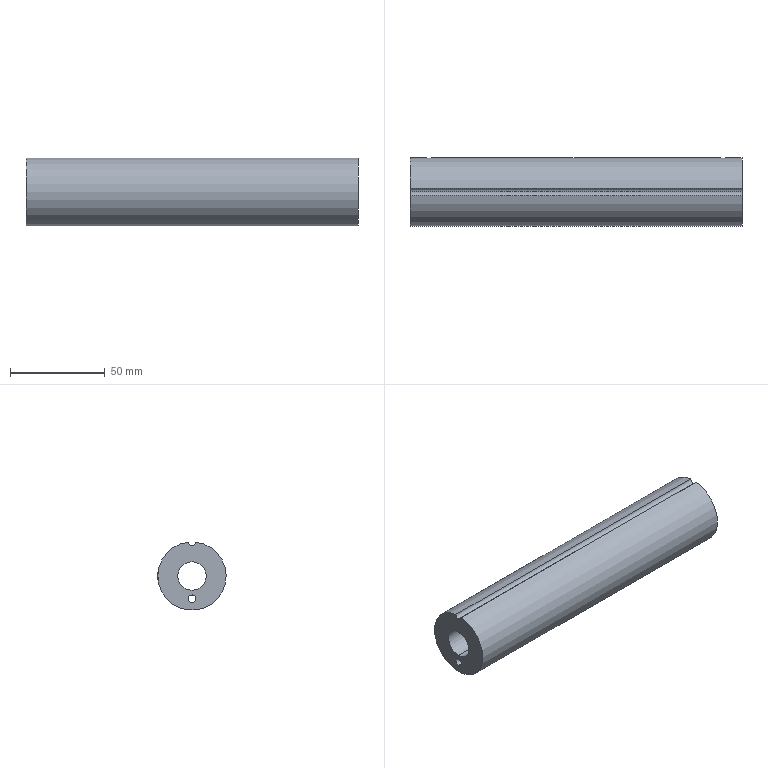Part | STEP file | MT-COMBO-119-S018 | 1 solid | 13 faces | box 175 x 36 x 35.889 mm | volume 143638 mm3 | cylinder 11 | plane 2 | commonest cylinder face diameters 4 x4 4.2 x4 15 x2 36 x1
STEP:
#1=CARTESIAN_POINT('',(-77.5,17.877,2.1));
#2=VERTEX_POINT('',#1);
#3=CARTESIAN_POINT('',(-77.5,17.877,-2.1));
#4=VERTEX_POINT('',#3);
#5=CARTESIAN_POINT('',(-77.5,17.877,2.1));
#6=CARTESIAN_POINT('',(-77.639,17.877,2.1));
#7=CARTESIAN_POINT('',(-77.775,17.879,2.086));
#8=CARTESIAN_POINT('',(-78.044,17.885,2.033));
#9=CARTESIAN_POINT('',(-78.177,17.889,1.993));
#10=CARTESIAN_POINT('',(-78.432,17.901,1.887));
#11=CARTESIAN_POINT('',(-78.552,17.908,1.823));
#12=CARTESIAN_POINT('',(-78.78,17.923,1.67));
#13=CARTESIAN_POINT('',(-78.888,17.931,1.582));
#14=CARTESIAN_POINT('',(-79.178,17.955,1.291));
#15=CARTESIAN_POINT('',(-79.335,17.971,1.057));
#16=CARTESIAN_POINT('',(-79.545,17.993,0.5521));
#17=CARTESIAN_POINT('',(-79.6,18.,0.2761));
#18=CARTESIAN_POINT('',(-79.6,18.,-0.1404));
#19=CARTESIAN_POINT('',(-79.586,17.998,-0.2769));
#20=CARTESIAN_POINT('',(-79.533,17.992,-0.5454));
#21=CARTESIAN_POINT('',(-79.492,17.988,-0.6788));
#22=CARTESIAN_POINT('',(-79.386,17.976,-0.9329));
#23=CARTESIAN_POINT('',(-79.322,17.97,-1.053));
#24=CARTESIAN_POINT('',(-79.169,17.955,-1.281));
#25=CARTESIAN_POINT('',(-79.081,17.947,-1.389));
#26=CARTESIAN_POINT('',(-78.79,17.923,-1.679));
#27=CARTESIAN_POINT('',(-78.556,17.906,-1.836));
#28=CARTESIAN_POINT('',(-78.051,17.884,-2.045));
#29=CARTESIAN_POINT('',(-77.774,17.877,-2.1));
#30=CARTESIAN_POINT('',(-77.5,17.877,-2.1));
#31=B_SPLINE_CURVE_WITH_KNOTS('',3,(#5,#6,#7,#8,#9,#10,#11,#12,#13,#14,#15,#16,#17,#18,#19,#20,#21,#22,#23,#24,#25,#26,#27,#28,#29,#30),.UNSPECIFIED.,.F.,.F.,(4,2,2,2,2,2,2,2,2,2,2,2,4),(0.009857,0.01027,0.01068,0.01109,0.0115,0.01232,0.01314,0.01355,0.01396,0.01437,0.01478,0.01561,0.01643),.UNSPECIFIED.);
#32=EDGE_CURVE('',#2,#4,#31,.T.);
#33=ORIENTED_EDGE('',*,*,#32,.F.);
#34=CARTESIAN_POINT('',(-77.5,7.2,2.1));
#35=VERTEX_POINT('',#34);
#36=CARTESIAN_POINT('',(-77.5,0.,2.1));
#37=DIRECTION('',(0.,-1.,0.));
#38=VECTOR('',#37,1000.);
#39=LINE('',#36,#38);
#40=EDGE_CURVE('',#2,#35,#39,.T.);
#41=ORIENTED_EDGE('',*,*,#40,.T.);
#42=CARTESIAN_POINT('',(-77.5,7.2,-2.1));
#43=VERTEX_POINT('',#42);
#44=CARTESIAN_POINT('',(-77.5,7.2,-2.1));
#45=CARTESIAN_POINT('',(-77.64,7.2,-2.1));
#46=CARTESIAN_POINT('',(-77.777,7.204,-2.086));
#47=CARTESIAN_POINT('',(-78.046,7.219,-2.032));
#48=CARTESIAN_POINT('',(-78.18,7.231,-1.992));
#49=CARTESIAN_POINT('',(-78.434,7.259,-1.886));
#50=CARTESIAN_POINT('',(-78.554,7.276,-1.822));
#51=CARTESIAN_POINT('',(-78.782,7.312,-1.669));
#52=CARTESIAN_POINT('',(-78.889,7.332,-1.581));
#53=CARTESIAN_POINT('',(-79.178,7.391,-1.292));
#54=CARTESIAN_POINT('',(-79.334,7.429,-1.059));
#55=CARTESIAN_POINT('',(-79.492,7.47,-0.68));
#56=CARTESIAN_POINT('',(-79.532,7.481,-0.5469));
#57=CARTESIAN_POINT('',(-79.586,7.496,-0.2754));
#58=CARTESIAN_POINT('',(-79.6,7.5,-0.1387));
#59=CARTESIAN_POINT('',(-79.6,7.5,0.1369));
#60=CARTESIAN_POINT('',(-79.586,7.496,0.2768));
#61=CARTESIAN_POINT('',(-79.532,7.481,0.5468));
#62=CARTESIAN_POINT('',(-79.492,7.47,0.678));
#63=CARTESIAN_POINT('',(-79.333,7.429,1.061));
#64=CARTESIAN_POINT('',(-79.179,7.391,1.291));
#65=CARTESIAN_POINT('',(-78.887,7.332,1.583));
#66=CARTESIAN_POINT('',(-78.782,7.312,1.669));
#67=CARTESIAN_POINT('',(-78.555,7.276,1.821));
#68=CARTESIAN_POINT('',(-78.432,7.259,1.887));
#69=CARTESIAN_POINT('',(-78.179,7.231,1.992));
#70=CARTESIAN_POINT('',(-78.048,7.22,2.032));
#71=CARTESIAN_POINT('',(-77.777,7.204,2.086));
#72=CARTESIAN_POINT('',(-77.637,7.2,2.1));
#73=CARTESIAN_POINT('',(-77.5,7.2,2.1));
#74=B_SPLINE_CURVE_WITH_KNOTS('',3,(#44,#45,#46,#47,#48,#49,#50,#51,#52,#53,#54,#55,#56,#57,#58,#59,#60,#61,#62,#63,#64,#65,#66,#67,#68,#69,#70,#71,#72,#73),.UNSPECIFIED.,.F.,.F.,(4,2,2,2,2,2,2,2,2,2,2,2,2,2,4),(0.,0.0004124,0.0008248,0.001237,0.00165,0.002474,0.002887,0.003299,0.003712,0.004124,0.004949,0.005361,0.005774,0.006186,0.006599),.UNSPECIFIED.);
#75=EDGE_CURVE('',#43,#35,#74,.T.);
#76=ORIENTED_EDGE('',*,*,#75,.F.);
#77=CARTESIAN_POINT('',(-77.5,0.,-2.1));
#78=DIRECTION('',(0.,-1.,0.));
#79=VECTOR('',#78,1000.);
#80=LINE('',#77,#79);
#81=EDGE_CURVE('',#4,#43,#80,.T.);
#82=ORIENTED_EDGE('',*,*,#81,.F.);
#83=EDGE_LOOP('',(#33,#41,#76,#82));
#84=FACE_OUTER_BOUND('',#83,.T.);
#85=CARTESIAN_POINT('',(-77.5,0.,0.));
#86=DIRECTION('',(0.,-1.,0.));
#87=DIRECTION('',(0.,0.,-1.));
#88=AXIS2_PLACEMENT_3D('',#85,#86,#87);
#89=CYLINDRICAL_SURFACE('',#88,2.1);
#90=ADVANCED_FACE('',(#84),#89,.F.);
#91=CARTESIAN_POINT('',(77.5,17.877,2.1));
#92=VERTEX_POINT('',#91);
#93=CARTESIAN_POINT('',(77.5,17.877,-2.1));
#94=VERTEX_POINT('',#93);
#95=CARTESIAN_POINT('',(77.5,17.877,2.1));
#96=CARTESIAN_POINT('',(77.361,17.877,2.1));
#97=CARTESIAN_POINT('',(77.225,17.879,2.086));
#98=CARTESIAN_POINT('',(76.956,17.885,2.033));
#99=CARTESIAN_POINT('',(76.823,17.889,1.993));
#100=CARTESIAN_POINT('',(76.568,17.901,1.887));
#101=CARTESIAN_POINT('',(76.448,17.908,1.823));
#102=CARTESIAN_POINT('',(76.22,17.923,1.67));
#103=CARTESIAN_POINT('',(76.112,17.931,1.582));
#104=CARTESIAN_POINT('',(75.822,17.955,1.291));
#105=CARTESIAN_POINT('',(75.665,17.971,1.057));
#106=CARTESIAN_POINT('',(75.455,17.993,0.5521));
#107=CARTESIAN_POINT('',(75.4,18.,0.2761));
#108=CARTESIAN_POINT('',(75.4,18.,-0.1404));
#109=CARTESIAN_POINT('',(75.414,17.998,-0.2769));
#110=CARTESIAN_POINT('',(75.467,17.992,-0.5454));
#111=CARTESIAN_POINT('',(75.508,17.988,-0.6788));
#112=CARTESIAN_POINT('',(75.614,17.976,-0.9329));
#113=CARTESIAN_POINT('',(75.678,17.97,-1.053));
#114=CARTESIAN_POINT('',(75.831,17.955,-1.281));
#115=CARTESIAN_POINT('',(75.919,17.947,-1.389));
#116=CARTESIAN_POINT('',(76.21,17.923,-1.679));
#117=CARTESIAN_POINT('',(76.444,17.906,-1.836));
#118=CARTESIAN_POINT('',(76.949,17.884,-2.045));
#119=CARTESIAN_POINT('',(77.226,17.877,-2.1));
#120=CARTESIAN_POINT('',(77.5,17.877,-2.1));
#121=B_SPLINE_CURVE_WITH_KNOTS('',3,(#95,#96,#97,#98,#99,#100,#101,#102,#103,#104,#105,#106,#107,#108,#109,#110,#111,#112,#113,#114,#115,#116,#117,#118,#119,#120),.UNSPECIFIED.,.F.,.F.,(4,2,2,2,2,2,2,2,2,2,2,2,4),(0.009857,0.01027,0.01068,0.01109,0.0115,0.01232,0.01314,0.01355,0.01396,0.01437,0.01478,0.01561,0.01643),.UNSPECIFIED.);
#122=EDGE_CURVE('',#92,#94,#121,.T.);
#123=ORIENTED_EDGE('',*,*,#122,.F.);
#124=CARTESIAN_POINT('',(77.5,7.2,2.1));
#125=VERTEX_POINT('',#124);
#126=CARTESIAN_POINT('',(77.5,0.,2.1));
#127=DIRECTION('',(0.,-1.,0.));
#128=VECTOR('',#127,1000.);
#129=LINE('',#126,#128);
#130=EDGE_CURVE('',#92,#125,#129,.T.);
#131=ORIENTED_EDGE('',*,*,#130,.T.);
#132=CARTESIAN_POINT('',(77.5,7.2,-2.1));
#133=VERTEX_POINT('',#132);
#134=CARTESIAN_POINT('',(77.5,7.2,-2.1));
#135=CARTESIAN_POINT('',(77.36,7.2,-2.1));
#136=CARTESIAN_POINT('',(77.223,7.204,-2.086));
#137=CARTESIAN_POINT('',(76.954,7.219,-2.032));
#138=CARTESIAN_POINT('',(76.82,7.231,-1.992));
#139=CARTESIAN_POINT('',(76.566,7.259,-1.886));
#140=CARTESIAN_POINT('',(76.446,7.276,-1.822));
#141=CARTESIAN_POINT('',(76.218,7.312,-1.669));
#142=CARTESIAN_POINT('',(76.111,7.332,-1.581));
#143=CARTESIAN_POINT('',(75.822,7.391,-1.292));
#144=CARTESIAN_POINT('',(75.666,7.429,-1.059));
#145=CARTESIAN_POINT('',(75.508,7.47,-0.68));
#146=CARTESIAN_POINT('',(75.468,7.481,-0.5469));
#147=CARTESIAN_POINT('',(75.414,7.496,-0.2754));
#148=CARTESIAN_POINT('',(75.4,7.5,-0.1387));
#149=CARTESIAN_POINT('',(75.4,7.5,0.1369));
#150=CARTESIAN_POINT('',(75.414,7.496,0.2768));
#151=CARTESIAN_POINT('',(75.468,7.481,0.5468));
#152=CARTESIAN_POINT('',(75.508,7.47,0.678));
#153=CARTESIAN_POINT('',(75.667,7.429,1.061));
#154=CARTESIAN_POINT('',(75.821,7.391,1.291));
#155=CARTESIAN_POINT('',(76.113,7.332,1.583));
#156=CARTESIAN_POINT('',(76.218,7.312,1.669));
#157=CARTESIAN_POINT('',(76.445,7.276,1.821));
#158=CARTESIAN_POINT('',(76.568,7.259,1.887));
#159=CARTESIAN_POINT('',(76.821,7.231,1.992));
#160=CARTESIAN_POINT('',(76.952,7.22,2.032));
#161=CARTESIAN_POINT('',(77.223,7.204,2.086));
#162=CARTESIAN_POINT('',(77.363,7.2,2.1));
#163=CARTESIAN_POINT('',(77.5,7.2,2.1));
#164=B_SPLINE_CURVE_WITH_KNOTS('',3,(#134,#135,#136,#137,#138,#139,#140,#141,#142,#143,#144,#145,#146,#147,#148,#149,#150,#151,#152,#153,#154,#155,#156,#157,#158,#159,#160,#161,#162,#163),.UNSPECIFIED.,.F.,.F.,(4,2,2,2,2,2,2,2,2,2,2,2,2,2,4),(0.,0.0004124,0.0008248,0.001237,0.00165,0.002474,0.002887,0.003299,0.003712,0.004124,0.004949,0.005361,0.005774,0.006186,0.006599),.UNSPECIFIED.);
#165=EDGE_CURVE('',#133,#125,#164,.T.);
#166=ORIENTED_EDGE('',*,*,#165,.F.);
#167=CARTESIAN_POINT('',(77.5,0.,-2.1));
#168=DIRECTION('',(0.,-1.,0.));
#169=VECTOR('',#168,1000.);
#170=LINE('',#167,#169);
#171=EDGE_CURVE('',#94,#133,#170,.T.);
#172=ORIENTED_EDGE('',*,*,#171,.F.);
#173=EDGE_LOOP('',(#123,#131,#166,#172));
#174=FACE_OUTER_BOUND('',#173,.T.);
#175=CARTESIAN_POINT('',(77.5,0.,0.));
#176=DIRECTION('',(0.,-1.,0.));
#177=DIRECTION('',(0.,0.,-1.));
#178=AXIS2_PLACEMENT_3D('',#175,#176,#177);
#179=CYLINDRICAL_SURFACE('',#178,2.1);
#180=ADVANCED_FACE('',(#174),#179,.F.);
#181=CARTESIAN_POINT('',(-87.5,0.,-10.));
#182=VERTEX_POINT('',#181);
#183=CARTESIAN_POINT('',(-87.5,0.,-14.));
#184=VERTEX_POINT('',#183);
#185=CARTESIAN_POINT('',(-87.5,0.,-12.));
#186=DIRECTION('',(1.,0.,0.));
#187=DIRECTION('',(0.,0.,-1.));
#188=AXIS2_PLACEMENT_3D('',#185,#186,#187);
#189=CIRCLE('',#188,2.);
#190=EDGE_CURVE('',#182,#184,#189,.T.);
#191=ORIENTED_EDGE('',*,*,#190,.F.);
#192=CARTESIAN_POINT('',(87.5,0.,-10.));
#193=VERTEX_POINT('',#192);
#194=CARTESIAN_POINT('',(87.5,0.,-10.));
#195=DIRECTION('',(1.,0.,0.));
#196=VECTOR('',#195,1000.);
#197=LINE('',#194,#196);
#198=EDGE_CURVE('',#182,#193,#197,.T.);
#199=ORIENTED_EDGE('',*,*,#198,.T.);
#200=CARTESIAN_POINT('',(87.5,0.,-14.));
#201=VERTEX_POINT('',#200);
#202=CARTESIAN_POINT('',(87.5,0.,-12.));
#203=DIRECTION('',(1.,0.,0.));
#204=DIRECTION('',(0.,0.,-1.));
#205=AXIS2_PLACEMENT_3D('',#202,#203,#204);
#206=CIRCLE('',#205,2.);
#207=EDGE_CURVE('',#193,#201,#206,.T.);
#208=ORIENTED_EDGE('',*,*,#207,.T.);
#209=CARTESIAN_POINT('',(87.5,0.,-14.));
#210=DIRECTION('',(1.,0.,0.));
#211=VECTOR('',#210,1000.);
#212=LINE('',#209,#211);
#213=EDGE_CURVE('',#184,#201,#212,.T.);
#214=ORIENTED_EDGE('',*,*,#213,.F.);
#215=EDGE_LOOP('',(#191,#199,#208,#214));
#216=FACE_OUTER_BOUND('',#215,.T.);
#217=CARTESIAN_POINT('',(87.5,0.,-12.));
#218=DIRECTION('',(1.,0.,0.));
#219=DIRECTION('',(0.,0.,-1.));
#220=AXIS2_PLACEMENT_3D('',#217,#218,#219);
#221=CYLINDRICAL_SURFACE('',#220,2.);
#222=ADVANCED_FACE('',(#216),#221,.F.);
#223=CARTESIAN_POINT('',(-87.5,0.,16.));
#224=VERTEX_POINT('',#223);
#225=CARTESIAN_POINT('',(-87.5,1.997,17.889));
#226=VERTEX_POINT('',#225);
#227=CARTESIAN_POINT('',(-87.5,0.,18.));
#228=DIRECTION('',(1.,0.,0.));
#229=DIRECTION('',(0.,0.,-1.));
#230=AXIS2_PLACEMENT_3D('',#227,#228,#229);
#231=CIRCLE('',#230,2.);
#232=EDGE_CURVE('',#224,#226,#231,.T.);
#233=ORIENTED_EDGE('',*,*,#232,.F.);
#234=CARTESIAN_POINT('',(87.5,0.,16.));
#235=VERTEX_POINT('',#234);
#236=CARTESIAN_POINT('',(87.5,0.,16.));
#237=DIRECTION('',(1.,0.,0.));
#238=VECTOR('',#237,1000.);
#239=LINE('',#236,#238);
#240=EDGE_CURVE('',#224,#235,#239,.T.);
#241=ORIENTED_EDGE('',*,*,#240,.T.);
#242=CARTESIAN_POINT('',(87.5,1.997,17.889));
#243=VERTEX_POINT('',#242);
#244=CARTESIAN_POINT('',(87.5,0.,18.));
#245=DIRECTION('',(-1.,0.,0.));
#246=DIRECTION('',(0.,0.,1.));
#247=AXIS2_PLACEMENT_3D('',#244,#245,#246);
#248=CIRCLE('',#247,2.);
#249=EDGE_CURVE('',#243,#235,#248,.T.);
#250=ORIENTED_EDGE('',*,*,#249,.F.);
#251=CARTESIAN_POINT('',(0.,1.997,17.889));
#252=DIRECTION('',(1.,0.,0.));
#253=VECTOR('',#252,1000.);
#254=LINE('',#251,#253);
#255=EDGE_CURVE('',#226,#243,#254,.T.);
#256=ORIENTED_EDGE('',*,*,#255,.F.);
#257=EDGE_LOOP('',(#233,#241,#250,#256));
#258=FACE_OUTER_BOUND('',#257,.T.);
#259=CARTESIAN_POINT('',(87.5,0.,18.));
#260=DIRECTION('',(1.,0.,0.));
#261=DIRECTION('',(0.,0.,-1.));
#262=AXIS2_PLACEMENT_3D('',#259,#260,#261);
#263=CYLINDRICAL_SURFACE('',#262,2.);
#264=ADVANCED_FACE('',(#258),#263,.F.);
#265=CARTESIAN_POINT('',(87.5,0.,-7.5));
#266=VERTEX_POINT('',#265);
#267=CARTESIAN_POINT('',(87.5,0.,7.5));
#268=VERTEX_POINT('',#267);
#269=CARTESIAN_POINT('',(87.5,0.,0.));
#270=DIRECTION('',(-1.,0.,0.));
#271=DIRECTION('',(0.,0.,1.));
#272=AXIS2_PLACEMENT_3D('',#269,#270,#271);
#273=CIRCLE('',#272,7.5);
#274=EDGE_CURVE('',#266,#268,#273,.T.);
#275=ORIENTED_EDGE('',*,*,#274,.F.);
#276=CARTESIAN_POINT('',(-87.5,0.,-7.5));
#277=VERTEX_POINT('',#276);
#278=CARTESIAN_POINT('',(0.,0.,-7.5));
#279=DIRECTION('',(-1.,0.,0.));
#280=VECTOR('',#279,1000.);
#281=LINE('',#278,#280);
#282=EDGE_CURVE('',#266,#277,#281,.T.);
#283=ORIENTED_EDGE('',*,*,#282,.T.);
#284=CARTESIAN_POINT('',(-87.5,0.,7.5));
#285=VERTEX_POINT('',#284);
#286=CARTESIAN_POINT('',(-87.5,0.,0.));
#287=DIRECTION('',(-1.,0.,0.));
#288=DIRECTION('',(0.,0.,1.));
#289=AXIS2_PLACEMENT_3D('',#286,#287,#288);
#290=CIRCLE('',#289,7.5);
#291=EDGE_CURVE('',#277,#285,#290,.T.);
#292=ORIENTED_EDGE('',*,*,#291,.T.);
#293=CARTESIAN_POINT('',(0.,0.,7.5));
#294=DIRECTION('',(-1.,0.,0.));
#295=VECTOR('',#294,1000.);
#296=LINE('',#293,#295);
#297=EDGE_CURVE('',#268,#285,#296,.T.);
#298=ORIENTED_EDGE('',*,*,#297,.F.);
#299=EDGE_LOOP('',(#275,#283,#292,#298));
#300=FACE_OUTER_BOUND('',#299,.T.);
#301=CARTESIAN_POINT('',(0.,0.,0.));
#302=DIRECTION('',(-1.,0.,0.));
#303=DIRECTION('',(0.,0.,1.));
#304=AXIS2_PLACEMENT_3D('',#301,#302,#303);
#305=CYLINDRICAL_SURFACE('',#304,7.5);
#306=ADVANCED_FACE('',(#300),#305,.F.);
#307=CARTESIAN_POINT('',(-77.5,17.877,-2.1));
#308=CARTESIAN_POINT('',(-77.363,17.877,-2.1));
#309=CARTESIAN_POINT('',(-77.224,17.879,-2.086));
#310=CARTESIAN_POINT('',(-76.954,17.885,-2.032));
#311=CARTESIAN_POINT('',(-76.823,17.889,-1.993));
#312=CARTESIAN_POINT('',(-76.569,17.901,-1.887));
#313=CARTESIAN_POINT('',(-76.446,17.908,-1.822));
#314=CARTESIAN_POINT('',(-76.219,17.923,-1.669));
#315=CARTESIAN_POINT('',(-76.113,17.931,-1.583));
#316=CARTESIAN_POINT('',(-75.917,17.947,-1.387));
#317=CARTESIAN_POINT('',(-75.83,17.955,-1.281));
#318=CARTESIAN_POINT('',(-75.678,17.97,-1.053));
#319=CARTESIAN_POINT('',(-75.612,17.976,-0.9303));
#320=CARTESIAN_POINT('',(-75.507,17.988,-0.676));
#321=CARTESIAN_POINT('',(-75.467,17.992,-0.545));
#322=CARTESIAN_POINT('',(-75.414,17.998,-0.2756));
#323=CARTESIAN_POINT('',(-75.4,18.,-0.1364));
#324=CARTESIAN_POINT('',(-75.4,18.,0.275));
#325=CARTESIAN_POINT('',(-75.455,17.993,0.5515));
#326=CARTESIAN_POINT('',(-75.665,17.971,1.057));
#327=CARTESIAN_POINT('',(-75.821,17.955,1.291));
#328=CARTESIAN_POINT('',(-76.112,17.931,1.582));
#329=CARTESIAN_POINT('',(-76.22,17.923,1.67));
#330=CARTESIAN_POINT('',(-76.448,17.908,1.823));
#331=CARTESIAN_POINT('',(-76.568,17.901,1.887));
#332=CARTESIAN_POINT('',(-76.823,17.889,1.993));
#333=CARTESIAN_POINT('',(-76.956,17.885,2.033));
#334=CARTESIAN_POINT('',(-77.225,17.879,2.086));
#335=CARTESIAN_POINT('',(-77.361,17.877,2.1));
#336=CARTESIAN_POINT('',(-77.5,17.877,2.1));
#337=B_SPLINE_CURVE_WITH_KNOTS('',3,(#307,#308,#309,#310,#311,#312,#313,#314,#315,#316,#317,#318,#319,#320,#321,#322,#323,#324,#325,#326,#327,#328,#329,#330,#331,#332,#333,#334,#335,#336),.UNSPECIFIED.,.F.,.F.,(4,2,2,2,2,2,2,2,2,2,2,2,2,2,4),(0.003286,0.003697,0.004108,0.004518,0.004929,0.00534,0.005751,0.006161,0.006572,0.007393,0.008215,0.008625,0.009036,0.009447,0.009857),.UNSPECIFIED.);
#338=EDGE_CURVE('',#4,#2,#337,.T.);
#339=ORIENTED_EDGE('',*,*,#338,.T.);
#340=ORIENTED_EDGE('',*,*,#32,.T.);
#341=EDGE_LOOP('',(#339,#340));
#342=FACE_BOUND('',#341,.T.);
#343=CARTESIAN_POINT('',(77.5,17.877,-2.1));
#344=CARTESIAN_POINT('',(77.637,17.877,-2.1));
#345=CARTESIAN_POINT('',(77.776,17.879,-2.086));
#346=CARTESIAN_POINT('',(78.046,17.885,-2.032));
#347=CARTESIAN_POINT('',(78.177,17.889,-1.993));
#348=CARTESIAN_POINT('',(78.431,17.901,-1.887));
#349=CARTESIAN_POINT('',(78.554,17.908,-1.822));
#350=CARTESIAN_POINT('',(78.781,17.923,-1.669));
#351=CARTESIAN_POINT('',(78.887,17.931,-1.583));
#352=CARTESIAN_POINT('',(79.083,17.947,-1.387));
#353=CARTESIAN_POINT('',(79.17,17.955,-1.281));
#354=CARTESIAN_POINT('',(79.322,17.97,-1.053));
#355=CARTESIAN_POINT('',(79.388,17.976,-0.9303));
#356=CARTESIAN_POINT('',(79.493,17.988,-0.676));
#357=CARTESIAN_POINT('',(79.533,17.992,-0.545));
#358=CARTESIAN_POINT('',(79.586,17.998,-0.2756));
#359=CARTESIAN_POINT('',(79.6,18.,-0.1364));
#360=CARTESIAN_POINT('',(79.6,18.,0.275));
#361=CARTESIAN_POINT('',(79.545,17.993,0.5515));
#362=CARTESIAN_POINT('',(79.335,17.971,1.057));
#363=CARTESIAN_POINT('',(79.179,17.955,1.291));
#364=CARTESIAN_POINT('',(78.888,17.931,1.582));
#365=CARTESIAN_POINT('',(78.78,17.923,1.67));
#366=CARTESIAN_POINT('',(78.552,17.908,1.823));
#367=CARTESIAN_POINT('',(78.432,17.901,1.887));
#368=CARTESIAN_POINT('',(78.177,17.889,1.993));
#369=CARTESIAN_POINT('',(78.044,17.885,2.033));
#370=CARTESIAN_POINT('',(77.775,17.879,2.086));
#371=CARTESIAN_POINT('',(77.639,17.877,2.1));
#372=CARTESIAN_POINT('',(77.5,17.877,2.1));
#373=B_SPLINE_CURVE_WITH_KNOTS('',3,(#343,#344,#345,#346,#347,#348,#349,#350,#351,#352,#353,#354,#355,#356,#357,#358,#359,#360,#361,#362,#363,#364,#365,#366,#367,#368,#369,#370,#371,#372),.UNSPECIFIED.,.F.,.F.,(4,2,2,2,2,2,2,2,2,2,2,2,2,2,4),(0.003286,0.003697,0.004108,0.004518,0.004929,0.00534,0.005751,0.006161,0.006572,0.007393,0.008215,0.008625,0.009036,0.009447,0.009857),.UNSPECIFIED.);
#374=EDGE_CURVE('',#94,#92,#373,.T.);
#375=ORIENTED_EDGE('',*,*,#374,.T.);
#376=ORIENTED_EDGE('',*,*,#122,.T.);
#377=EDGE_LOOP('',(#375,#376));
#378=FACE_BOUND('',#377,.T.);
#379=CARTESIAN_POINT('',(-87.5,-1.997,17.889));
#380=VERTEX_POINT('',#379);
#381=CARTESIAN_POINT('',(-87.5,0.,0.));
#382=DIRECTION('',(-1.,0.,0.));
#383=DIRECTION('',(0.,0.,1.));
#384=AXIS2_PLACEMENT_3D('',#381,#382,#383);
#385=CIRCLE('',#384,18.);
#386=EDGE_CURVE('',#226,#380,#385,.T.);
#387=ORIENTED_EDGE('',*,*,#386,.F.);
#388=ORIENTED_EDGE('',*,*,#255,.T.);
#389=CARTESIAN_POINT('',(87.5,-1.997,17.889));
#390=VERTEX_POINT('',#389);
#391=CARTESIAN_POINT('',(87.5,0.,0.));
#392=DIRECTION('',(-1.,0.,0.));
#393=DIRECTION('',(0.,0.,1.));
#394=AXIS2_PLACEMENT_3D('',#391,#392,#393);
#395=CIRCLE('',#394,18.);
#396=EDGE_CURVE('',#243,#390,#395,.T.);
#397=ORIENTED_EDGE('',*,*,#396,.T.);
#398=CARTESIAN_POINT('',(0.,-1.997,17.889));
#399=DIRECTION('',(-1.,0.,0.));
#400=VECTOR('',#399,1000.);
#401=LINE('',#398,#400);
#402=EDGE_CURVE('',#390,#380,#401,.T.);
#403=ORIENTED_EDGE('',*,*,#402,.T.);
#404=EDGE_LOOP('',(#387,#388,#397,#403));
#405=FACE_OUTER_BOUND('',#404,.T.);
#406=CARTESIAN_POINT('',(0.,0.,0.));
#407=DIRECTION('',(-1.,0.,0.));
#408=DIRECTION('',(0.,0.,1.));
#409=AXIS2_PLACEMENT_3D('',#406,#407,#408);
#410=CYLINDRICAL_SURFACE('',#409,18.);
#411=ADVANCED_FACE('',(#342,#378,#405),#410,.T.);
#412=CARTESIAN_POINT('',(-87.5,0.,-12.));
#413=DIRECTION('',(1.,0.,0.));
#414=DIRECTION('',(0.,0.,-1.));
#415=AXIS2_PLACEMENT_3D('',#412,#413,#414);
#416=CIRCLE('',#415,2.);
#417=EDGE_CURVE('',#184,#182,#416,.T.);
#418=ORIENTED_EDGE('',*,*,#417,.T.);
#419=ORIENTED_EDGE('',*,*,#190,.T.);
#420=EDGE_LOOP('',(#418,#419));
#421=FACE_BOUND('',#420,.T.);
#422=CARTESIAN_POINT('',(-87.5,0.,0.));
#423=DIRECTION('',(-1.,0.,0.));
#424=DIRECTION('',(0.,0.,1.));
#425=AXIS2_PLACEMENT_3D('',#422,#423,#424);
#426=CIRCLE('',#425,7.5);
#427=EDGE_CURVE('',#285,#277,#426,.T.);
#428=ORIENTED_EDGE('',*,*,#427,.F.);
#429=ORIENTED_EDGE('',*,*,#291,.F.);
#430=EDGE_LOOP('',(#428,#429));
#431=FACE_BOUND('',#430,.T.);
#432=ORIENTED_EDGE('',*,*,#386,.T.);
#433=CARTESIAN_POINT('',(-87.5,0.,18.));
#434=DIRECTION('',(1.,0.,0.));
#435=DIRECTION('',(0.,0.,-1.));
#436=AXIS2_PLACEMENT_3D('',#433,#434,#435);
#437=CIRCLE('',#436,2.);
#438=EDGE_CURVE('',#380,#224,#437,.T.);
#439=ORIENTED_EDGE('',*,*,#438,.T.);
#440=ORIENTED_EDGE('',*,*,#232,.T.);
#441=EDGE_LOOP('',(#432,#439,#440));
#442=FACE_OUTER_BOUND('',#441,.T.);
#443=CARTESIAN_POINT('',(-87.5,18.,0.));
#444=DIRECTION('',(1.,0.,0.));
#445=DIRECTION('',(0.,0.,-1.));
#446=AXIS2_PLACEMENT_3D('',#443,#444,#445);
#447=PLANE('',#446);
#448=ADVANCED_FACE('',(#421,#431,#442),#447,.F.);
#449=ORIENTED_EDGE('',*,*,#282,.F.);
#450=CARTESIAN_POINT('',(87.5,0.,0.));
#451=DIRECTION('',(-1.,0.,0.));
#452=DIRECTION('',(0.,0.,1.));
#453=AXIS2_PLACEMENT_3D('',#450,#451,#452);
#454=CIRCLE('',#453,7.5);
#455=EDGE_CURVE('',#268,#266,#454,.T.);
#456=ORIENTED_EDGE('',*,*,#455,.F.);
#457=ORIENTED_EDGE('',*,*,#297,.T.);
#458=ORIENTED_EDGE('',*,*,#427,.T.);
#459=EDGE_LOOP('',(#449,#456,#457,#458));
#460=FACE_OUTER_BOUND('',#459,.T.);
#461=ORIENTED_EDGE('',*,*,#75,.T.);
#462=CARTESIAN_POINT('',(-77.5,7.2,2.1));
#463=CARTESIAN_POINT('',(-77.225,7.2,2.1));
#464=CARTESIAN_POINT('',(-76.948,7.217,2.044));
#465=CARTESIAN_POINT('',(-76.568,7.259,1.887));
#466=CARTESIAN_POINT('',(-76.445,7.276,1.821));
#467=CARTESIAN_POINT('',(-76.218,7.312,1.669));
#468=CARTESIAN_POINT('',(-76.113,7.332,1.582));
#469=CARTESIAN_POINT('',(-75.919,7.371,1.389));
#470=CARTESIAN_POINT('',(-75.831,7.391,1.282));
#471=CARTESIAN_POINT('',(-75.679,7.426,1.055));
#472=CARTESIAN_POINT('',(-75.614,7.443,0.9346));
#473=CARTESIAN_POINT('',(-75.508,7.47,0.6786));
#474=CARTESIAN_POINT('',(-75.468,7.481,0.547));
#475=CARTESIAN_POINT('',(-75.414,7.496,0.278));
#476=CARTESIAN_POINT('',(-75.4,7.5,0.1388));
#477=CARTESIAN_POINT('',(-75.4,7.5,-0.1381));
#478=CARTESIAN_POINT('',(-75.414,7.496,-0.2749));
#479=CARTESIAN_POINT('',(-75.467,7.481,-0.5451));
#480=CARTESIAN_POINT('',(-75.508,7.47,-0.6791));
#481=CARTESIAN_POINT('',(-75.666,7.429,-1.059));
#482=CARTESIAN_POINT('',(-75.822,7.391,-1.292));
#483=CARTESIAN_POINT('',(-76.111,7.332,-1.581));
#484=CARTESIAN_POINT('',(-76.218,7.312,-1.669));
#485=CARTESIAN_POINT('',(-76.446,7.276,-1.821));
#486=CARTESIAN_POINT('',(-76.566,7.259,-1.886));
#487=CARTESIAN_POINT('',(-76.819,7.231,-1.991));
#488=CARTESIAN_POINT('',(-76.953,7.219,-2.032));
#489=CARTESIAN_POINT('',(-77.223,7.204,-2.086));
#490=CARTESIAN_POINT('',(-77.361,7.2,-2.1));
#491=CARTESIAN_POINT('',(-77.5,7.2,-2.1));
#492=B_SPLINE_CURVE_WITH_KNOTS('',3,(#462,#463,#464,#465,#466,#467,#468,#469,#470,#471,#472,#473,#474,#475,#476,#477,#478,#479,#480,#481,#482,#483,#484,#485,#486,#487,#488,#489,#490,#491),.UNSPECIFIED.,.F.,.F.,(4,2,2,2,2,2,2,2,2,2,2,2,2,2,4),(0.006599,0.007423,0.007836,0.008248,0.00866,0.009072,0.009485,0.009897,0.01031,0.01072,0.01155,0.01196,0.01237,0.01278,0.0132),.UNSPECIFIED.);
#493=EDGE_CURVE('',#35,#43,#492,.T.);
#494=ORIENTED_EDGE('',*,*,#493,.T.);
#495=EDGE_LOOP('',(#461,#494));
#496=FACE_BOUND('',#495,.T.);
#497=ORIENTED_EDGE('',*,*,#165,.T.);
#498=CARTESIAN_POINT('',(77.5,7.2,2.1));
#499=CARTESIAN_POINT('',(77.775,7.2,2.1));
#500=CARTESIAN_POINT('',(78.052,7.217,2.044));
#501=CARTESIAN_POINT('',(78.432,7.259,1.887));
#502=CARTESIAN_POINT('',(78.555,7.276,1.821));
#503=CARTESIAN_POINT('',(78.782,7.312,1.669));
#504=CARTESIAN_POINT('',(78.887,7.332,1.582));
#505=CARTESIAN_POINT('',(79.081,7.371,1.389));
#506=CARTESIAN_POINT('',(79.169,7.391,1.282));
#507=CARTESIAN_POINT('',(79.321,7.426,1.055));
#508=CARTESIAN_POINT('',(79.386,7.443,0.9346));
#509=CARTESIAN_POINT('',(79.492,7.47,0.6786));
#510=CARTESIAN_POINT('',(79.532,7.481,0.547));
#511=CARTESIAN_POINT('',(79.586,7.496,0.278));
#512=CARTESIAN_POINT('',(79.6,7.5,0.1388));
#513=CARTESIAN_POINT('',(79.6,7.5,-0.1381));
#514=CARTESIAN_POINT('',(79.586,7.496,-0.2749));
#515=CARTESIAN_POINT('',(79.533,7.481,-0.5451));
#516=CARTESIAN_POINT('',(79.492,7.47,-0.6791));
#517=CARTESIAN_POINT('',(79.334,7.429,-1.059));
#518=CARTESIAN_POINT('',(79.178,7.391,-1.292));
#519=CARTESIAN_POINT('',(78.889,7.332,-1.581));
#520=CARTESIAN_POINT('',(78.782,7.312,-1.669));
#521=CARTESIAN_POINT('',(78.554,7.276,-1.821));
#522=CARTESIAN_POINT('',(78.434,7.259,-1.886));
#523=CARTESIAN_POINT('',(78.181,7.231,-1.991));
#524=CARTESIAN_POINT('',(78.047,7.219,-2.032));
#525=CARTESIAN_POINT('',(77.777,7.204,-2.086));
#526=CARTESIAN_POINT('',(77.639,7.2,-2.1));
#527=CARTESIAN_POINT('',(77.5,7.2,-2.1));
#528=B_SPLINE_CURVE_WITH_KNOTS('',3,(#498,#499,#500,#501,#502,#503,#504,#505,#506,#507,#508,#509,#510,#511,#512,#513,#514,#515,#516,#517,#518,#519,#520,#521,#522,#523,#524,#525,#526,#527),.UNSPECIFIED.,.F.,.F.,(4,2,2,2,2,2,2,2,2,2,2,2,2,2,4),(0.006599,0.007423,0.007836,0.008248,0.00866,0.009072,0.009485,0.009897,0.01031,0.01072,0.01155,0.01196,0.01237,0.01278,0.0132),.UNSPECIFIED.);
#529=EDGE_CURVE('',#125,#133,#528,.T.);
#530=ORIENTED_EDGE('',*,*,#529,.T.);
#531=EDGE_LOOP('',(#497,#530));
#532=FACE_BOUND('',#531,.T.);
#533=CARTESIAN_POINT('',(0.,0.,0.));
#534=DIRECTION('',(-1.,0.,0.));
#535=DIRECTION('',(0.,0.,1.));
#536=AXIS2_PLACEMENT_3D('',#533,#534,#535);
#537=CYLINDRICAL_SURFACE('',#536,7.5);
#538=ADVANCED_FACE('',(#460,#496,#532),#537,.F.);
#539=CARTESIAN_POINT('',(87.5,0.,-12.));
#540=DIRECTION('',(1.,0.,0.));
#541=DIRECTION('',(0.,0.,-1.));
#542=AXIS2_PLACEMENT_3D('',#539,#540,#541);
#543=CIRCLE('',#542,2.);
#544=EDGE_CURVE('',#201,#193,#543,.T.);
#545=ORIENTED_EDGE('',*,*,#544,.F.);
#546=ORIENTED_EDGE('',*,*,#207,.F.);
#547=EDGE_LOOP('',(#545,#546));
#548=FACE_BOUND('',#547,.T.);
#549=ORIENTED_EDGE('',*,*,#396,.F.);
#550=ORIENTED_EDGE('',*,*,#249,.T.);
#551=CARTESIAN_POINT('',(87.5,0.,18.));
#552=DIRECTION('',(-1.,0.,0.));
#553=DIRECTION('',(0.,0.,1.));
#554=AXIS2_PLACEMENT_3D('',#551,#552,#553);
#555=CIRCLE('',#554,2.);
#556=EDGE_CURVE('',#235,#390,#555,.T.);
#557=ORIENTED_EDGE('',*,*,#556,.T.);
#558=EDGE_LOOP('',(#549,#550,#557));
#559=FACE_OUTER_BOUND('',#558,.T.);
#560=ORIENTED_EDGE('',*,*,#455,.T.);
#561=ORIENTED_EDGE('',*,*,#274,.T.);
#562=EDGE_LOOP('',(#560,#561));
#563=FACE_BOUND('',#562,.T.);
#564=CARTESIAN_POINT('',(87.5,7.5,0.));
#565=DIRECTION('',(-1.,0.,0.));
#566=DIRECTION('',(0.,0.,1.));
#567=AXIS2_PLACEMENT_3D('',#564,#565,#566);
#568=PLANE('',#567);
#569=ADVANCED_FACE('',(#548,#559,#563),#568,.F.);
#570=ORIENTED_EDGE('',*,*,#240,.F.);
#571=ORIENTED_EDGE('',*,*,#438,.F.);
#572=ORIENTED_EDGE('',*,*,#402,.F.);
#573=ORIENTED_EDGE('',*,*,#556,.F.);
#574=EDGE_LOOP('',(#570,#571,#572,#573));
#575=FACE_OUTER_BOUND('',#574,.T.);
#576=CARTESIAN_POINT('',(87.5,0.,18.));
#577=DIRECTION('',(1.,0.,0.));
#578=DIRECTION('',(0.,0.,-1.));
#579=AXIS2_PLACEMENT_3D('',#576,#577,#578);
#580=CYLINDRICAL_SURFACE('',#579,2.);
#581=ADVANCED_FACE('',(#575),#580,.F.);
#582=ORIENTED_EDGE('',*,*,#198,.F.);
#583=ORIENTED_EDGE('',*,*,#417,.F.);
#584=ORIENTED_EDGE('',*,*,#213,.T.);
#585=ORIENTED_EDGE('',*,*,#544,.T.);
#586=EDGE_LOOP('',(#582,#583,#584,#585));
#587=FACE_OUTER_BOUND('',#586,.T.);
#588=CARTESIAN_POINT('',(87.5,0.,-12.));
#589=DIRECTION('',(1.,0.,0.));
#590=DIRECTION('',(0.,0.,-1.));
#591=AXIS2_PLACEMENT_3D('',#588,#589,#590);
#592=CYLINDRICAL_SURFACE('',#591,2.);
#593=ADVANCED_FACE('',(#587),#592,.F.);
#594=ORIENTED_EDGE('',*,*,#130,.F.);
#595=ORIENTED_EDGE('',*,*,#374,.F.);
#596=ORIENTED_EDGE('',*,*,#171,.T.);
#597=ORIENTED_EDGE('',*,*,#529,.F.);
#598=EDGE_LOOP('',(#594,#595,#596,#597));
#599=FACE_OUTER_BOUND('',#598,.T.);
#600=CARTESIAN_POINT('',(77.5,0.,0.));
#601=DIRECTION('',(0.,-1.,0.));
#602=DIRECTION('',(0.,0.,-1.));
#603=AXIS2_PLACEMENT_3D('',#600,#601,#602);
#604=CYLINDRICAL_SURFACE('',#603,2.1);
#605=ADVANCED_FACE('',(#599),#604,.F.);
#606=ORIENTED_EDGE('',*,*,#40,.F.);
#607=ORIENTED_EDGE('',*,*,#338,.F.);
#608=ORIENTED_EDGE('',*,*,#81,.T.);
#609=ORIENTED_EDGE('',*,*,#493,.F.);
#610=EDGE_LOOP('',(#606,#607,#608,#609));
#611=FACE_OUTER_BOUND('',#610,.T.);
#612=CARTESIAN_POINT('',(-77.5,0.,0.));
#613=DIRECTION('',(0.,-1.,0.));
#614=DIRECTION('',(0.,0.,-1.));
#615=AXIS2_PLACEMENT_3D('',#612,#613,#614);
#616=CYLINDRICAL_SURFACE('',#615,2.1);
#617=ADVANCED_FACE('',(#611),#616,.F.);
#618=CLOSED_SHELL('',(#90,#180,#222,#264,#306,#411,#448,#538,#569,#581,#593,#605,#617));
#619=MANIFOLD_SOLID_BREP('',#618);
#620=CARTESIAN_POINT('',(0.,0.,0.));
#621=DIRECTION('',(0.,0.,1.));
#622=DIRECTION('',(1.,0.,0.));
#623=AXIS2_PLACEMENT_3D('',#620,#621,#622);
#624=(LENGTH_UNIT()NAMED_UNIT(*)SI_UNIT(.MILLI.,.METRE.));
#625=UNCERTAINTY_MEASURE_WITH_UNIT(LENGTH_MEASURE(0.00001),#624,'','');
#626=(NAMED_UNIT(*)PLANE_ANGLE_UNIT()SI_UNIT($,.RADIAN.));
#627=(NAMED_UNIT(*)SI_UNIT($,.STERADIAN.)SOLID_ANGLE_UNIT());
#628=(GEOMETRIC_REPRESENTATION_CONTEXT(3)GLOBAL_UNCERTAINTY_ASSIGNED_CONTEXT((#625))GLOBAL_UNIT_ASSIGNED_CONTEXT((#624,#626,#627))REPRESENTATION_CONTEXT('',''));
#629=ADVANCED_BREP_SHAPE_REPRESENTATION('',(#619,#623),#628);